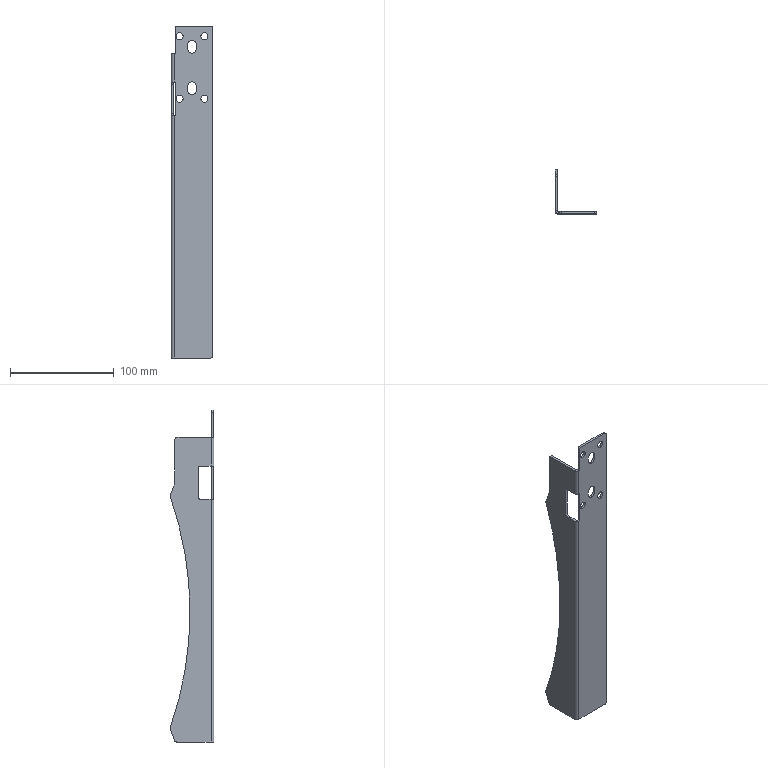Part | 1 solid | 59 faces | box 40 x 42.274 x 320 mm | volume 40668 mm3 | cylinder 31 | plane 28 | commonest cylinder face diameters 4 x12 6.8 x8 8.4 x6 1.48 x2 5.48 x2 668.4 x1